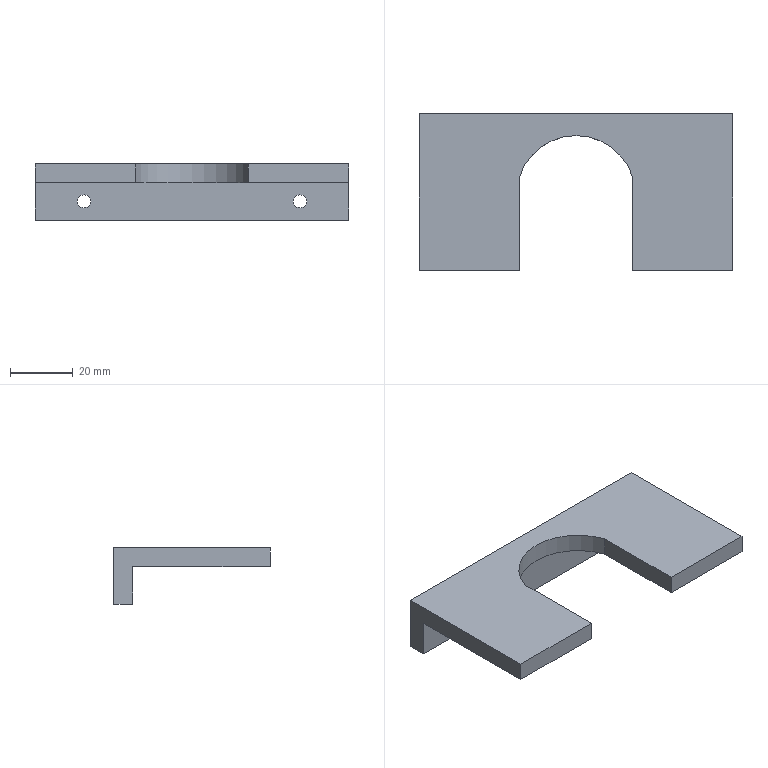Part | STEP file | Tube locking block SGN-6-04 | 1 solid | 16 faces | box 100 x 50 x 18 mm | volume 28496 mm3 | plane 11 | cylinder 5 | commonest cylinder face diameters 4.2 x4 38 x1
STEP:
#1=CARTESIAN_POINT('',(0.,0.,0.));
#2=DIRECTION('',(0.,0.,1.));
#3=DIRECTION('',(1.,0.,0.));
#4=AXIS2_PLACEMENT_3D('',#1,#2,#3);
#5=CARTESIAN_POINT('',(-34.5,19.,-3.9));
#6=VERTEX_POINT('',#5);
#7=CARTESIAN_POINT('',(-34.5,25.,-3.9));
#8=VERTEX_POINT('',#7);
#9=CARTESIAN_POINT('',(-34.5,25.,-3.9));
#10=DIRECTION('',(0.,1.,0.));
#11=VECTOR('',#10,1.);
#12=LINE('',#9,#11);
#13=CARTESIAN_POINT('',(-34.5,25.,-6.));
#14=DIRECTION('',(0.,1.,0.));
#15=DIRECTION('',(0.,0.,1.));
#16=AXIS2_PLACEMENT_3D('',#13,#14,#15);
#17=CYLINDRICAL_SURFACE('',#16,2.1);
#18=CARTESIAN_POINT('',(6.283,0.));
#19=DIRECTION('',(0.,1.));
#20=VECTOR('',#19,1.);
#21=LINE('',#18,#20);
#22=(GEOMETRIC_REPRESENTATION_CONTEXT(2)PARAMETRIC_REPRESENTATION_CONTEXT()REPRESENTATION_CONTEXT('',''));
#23=DEFINITIONAL_REPRESENTATION('',(#21),#22);
#24=PCURVE('',#17,#23);
#25=CARTESIAN_POINT('',(-34.5,25.,-6.));
#26=DIRECTION('',(0.,1.,0.));
#27=DIRECTION('',(0.,0.,1.));
#28=AXIS2_PLACEMENT_3D('',#25,#26,#27);
#29=CYLINDRICAL_SURFACE('',#28,2.1);
#30=CARTESIAN_POINT('',(0.,0.));
#31=DIRECTION('',(0.,1.));
#32=VECTOR('',#31,1.);
#33=LINE('',#30,#32);
#34=(GEOMETRIC_REPRESENTATION_CONTEXT(2)PARAMETRIC_REPRESENTATION_CONTEXT()REPRESENTATION_CONTEXT('',''));
#35=DEFINITIONAL_REPRESENTATION('',(#33),#34);
#36=PCURVE('',#29,#35);
#37=SURFACE_CURVE('',#12,(#24,#36),.PCURVE_S1.);
#38=EDGE_CURVE('',#6,#8,#37,.T.);
#39=ORIENTED_EDGE('',*,*,#38,.T.);
#40=CARTESIAN_POINT('',(-34.5,25.,-8.1));
#41=VERTEX_POINT('',#40);
#42=CARTESIAN_POINT('',(-34.5,25.,-6.));
#43=DIRECTION('',(0.,1.,0.));
#44=DIRECTION('',(0.,0.,1.));
#45=AXIS2_PLACEMENT_3D('',#42,#43,#44);
#46=CIRCLE('',#45,2.1);
#47=CARTESIAN_POINT('',(0.,0.));
#48=DIRECTION('',(1.,0.));
#49=VECTOR('',#48,1.);
#50=LINE('',#47,#49);
#51=(GEOMETRIC_REPRESENTATION_CONTEXT(2)PARAMETRIC_REPRESENTATION_CONTEXT()REPRESENTATION_CONTEXT('',''));
#52=DEFINITIONAL_REPRESENTATION('',(#50),#51);
#53=PCURVE('',#17,#52);
#54=CARTESIAN_POINT('',(-50.,25.,6.));
#55=DIRECTION('',(0.,-1.,0.));
#56=DIRECTION('',(1.,0.,0.));
#57=AXIS2_PLACEMENT_3D('',#54,#55,#56);
#58=PLANE('',#57);
#59=CARTESIAN_POINT('',(15.5,-9.9));
#60=CARTESIAN_POINT('',(19.137,-9.9));
#61=CARTESIAN_POINT('',(17.319,-13.05));
#62=CARTESIAN_POINT('',(15.5,-16.2));
#63=CARTESIAN_POINT('',(13.681,-13.05));
#64=CARTESIAN_POINT('',(11.863,-9.9));
#65=CARTESIAN_POINT('',(15.5,-9.9));
#66=(BOUNDED_CURVE()B_SPLINE_CURVE(2,(#59,#60,#61,#62,#63,#64,#65),.UNSPECIFIED.,.T.,.F.)B_SPLINE_CURVE_WITH_KNOTS((1,2,2,2,2,1),(-2.094,0.,2.094,4.189,6.283,8.378),.UNSPECIFIED.)CURVE()GEOMETRIC_REPRESENTATION_ITEM()RATIONAL_B_SPLINE_CURVE((1.,0.5,1.,0.5,1.,0.5,1.))REPRESENTATION_ITEM(''));
#67=(GEOMETRIC_REPRESENTATION_CONTEXT(2)PARAMETRIC_REPRESENTATION_CONTEXT()REPRESENTATION_CONTEXT('',''));
#68=DEFINITIONAL_REPRESENTATION('',(#66),#67);
#69=PCURVE('',#58,#68);
#70=SURFACE_CURVE('',#46,(#53,#69),.PCURVE_S1.);
#71=EDGE_CURVE('',#41,#8,#70,.T.);
#72=ORIENTED_EDGE('',*,*,#71,.F.);
#73=CARTESIAN_POINT('',(-34.5,19.,-8.1));
#74=VERTEX_POINT('',#73);
#75=CARTESIAN_POINT('',(-34.5,25.,-8.1));
#76=DIRECTION('',(0.,1.,0.));
#77=VECTOR('',#76,1.);
#78=LINE('',#75,#77);
#79=CARTESIAN_POINT('',(3.142,0.));
#80=DIRECTION('',(0.,1.));
#81=VECTOR('',#80,1.);
#82=LINE('',#79,#81);
#83=(GEOMETRIC_REPRESENTATION_CONTEXT(2)PARAMETRIC_REPRESENTATION_CONTEXT()REPRESENTATION_CONTEXT('',''));
#84=DEFINITIONAL_REPRESENTATION('',(#82),#83);
#85=PCURVE('',#17,#84);
#86=CARTESIAN_POINT('',(3.142,0.));
#87=DIRECTION('',(0.,1.));
#88=VECTOR('',#87,1.);
#89=LINE('',#86,#88);
#90=(GEOMETRIC_REPRESENTATION_CONTEXT(2)PARAMETRIC_REPRESENTATION_CONTEXT()REPRESENTATION_CONTEXT('',''));
#91=DEFINITIONAL_REPRESENTATION('',(#89),#90);
#92=PCURVE('',#29,#91);
#93=SURFACE_CURVE('',#78,(#85,#92),.PCURVE_S1.);
#94=EDGE_CURVE('',#74,#41,#93,.T.);
#95=ORIENTED_EDGE('',*,*,#94,.F.);
#96=CARTESIAN_POINT('',(-34.5,19.,-6.));
#97=DIRECTION('',(0.,1.,0.));
#98=DIRECTION('',(0.,0.,1.));
#99=AXIS2_PLACEMENT_3D('',#96,#97,#98);
#100=CIRCLE('',#99,2.1);
#101=CARTESIAN_POINT('',(0.,-6.));
#102=DIRECTION('',(1.,0.));
#103=VECTOR('',#102,1.);
#104=LINE('',#101,#103);
#105=(GEOMETRIC_REPRESENTATION_CONTEXT(2)PARAMETRIC_REPRESENTATION_CONTEXT()REPRESENTATION_CONTEXT('',''));
#106=DEFINITIONAL_REPRESENTATION('',(#104),#105);
#107=PCURVE('',#17,#106);
#108=CARTESIAN_POINT('',(50.,19.,-12.));
#109=DIRECTION('',(0.,1.,0.));
#110=DIRECTION('',(0.,0.,1.));
#111=AXIS2_PLACEMENT_3D('',#108,#109,#110);
#112=PLANE('',#111);
#113=CARTESIAN_POINT('',(6.,-84.5));
#114=DIRECTION('',(1.,0.));
#115=AXIS2_PLACEMENT_2D('',#113,#114);
#116=CIRCLE('',#115,2.1);
#117=(GEOMETRIC_REPRESENTATION_CONTEXT(2)PARAMETRIC_REPRESENTATION_CONTEXT()REPRESENTATION_CONTEXT('',''));
#118=DEFINITIONAL_REPRESENTATION('',(#116),#117);
#119=PCURVE('',#112,#118);
#120=SURFACE_CURVE('',#100,(#107,#119),.PCURVE_S1.);
#121=EDGE_CURVE('',#74,#6,#120,.T.);
#122=ORIENTED_EDGE('',*,*,#121,.T.);
#123=EDGE_LOOP('',(#39,#72,#95,#122));
#124=FACE_BOUND('',#123,.F.);
#125=ADVANCED_FACE('',(#124),#17,.F.);
#126=CARTESIAN_POINT('',(34.5,19.,-3.9));
#127=VERTEX_POINT('',#126);
#128=CARTESIAN_POINT('',(34.5,25.,-3.9));
#129=VERTEX_POINT('',#128);
#130=CARTESIAN_POINT('',(34.5,25.,-3.9));
#131=DIRECTION('',(0.,1.,0.));
#132=VECTOR('',#131,1.);
#133=LINE('',#130,#132);
#134=CARTESIAN_POINT('',(34.5,25.,-6.));
#135=DIRECTION('',(0.,1.,0.));
#136=DIRECTION('',(0.,0.,1.));
#137=AXIS2_PLACEMENT_3D('',#134,#135,#136);
#138=CYLINDRICAL_SURFACE('',#137,2.1);
#139=CARTESIAN_POINT('',(6.283,0.));
#140=DIRECTION('',(0.,1.));
#141=VECTOR('',#140,1.);
#142=LINE('',#139,#141);
#143=(GEOMETRIC_REPRESENTATION_CONTEXT(2)PARAMETRIC_REPRESENTATION_CONTEXT()REPRESENTATION_CONTEXT('',''));
#144=DEFINITIONAL_REPRESENTATION('',(#142),#143);
#145=PCURVE('',#138,#144);
#146=CARTESIAN_POINT('',(34.5,25.,-6.));
#147=DIRECTION('',(0.,1.,0.));
#148=DIRECTION('',(0.,0.,1.));
#149=AXIS2_PLACEMENT_3D('',#146,#147,#148);
#150=CYLINDRICAL_SURFACE('',#149,2.1);
#151=CARTESIAN_POINT('',(0.,0.));
#152=DIRECTION('',(0.,1.));
#153=VECTOR('',#152,1.);
#154=LINE('',#151,#153);
#155=(GEOMETRIC_REPRESENTATION_CONTEXT(2)PARAMETRIC_REPRESENTATION_CONTEXT()REPRESENTATION_CONTEXT('',''));
#156=DEFINITIONAL_REPRESENTATION('',(#154),#155);
#157=PCURVE('',#150,#156);
#158=SURFACE_CURVE('',#133,(#145,#157),.PCURVE_S1.);
#159=EDGE_CURVE('',#127,#129,#158,.T.);
#160=ORIENTED_EDGE('',*,*,#159,.T.);
#161=CARTESIAN_POINT('',(34.5,25.,-8.1));
#162=VERTEX_POINT('',#161);
#163=CARTESIAN_POINT('',(34.5,25.,-6.));
#164=DIRECTION('',(0.,1.,0.));
#165=DIRECTION('',(0.,0.,1.));
#166=AXIS2_PLACEMENT_3D('',#163,#164,#165);
#167=CIRCLE('',#166,2.1);
#168=CARTESIAN_POINT('',(0.,0.));
#169=DIRECTION('',(1.,0.));
#170=VECTOR('',#169,1.);
#171=LINE('',#168,#170);
#172=(GEOMETRIC_REPRESENTATION_CONTEXT(2)PARAMETRIC_REPRESENTATION_CONTEXT()REPRESENTATION_CONTEXT('',''));
#173=DEFINITIONAL_REPRESENTATION('',(#171),#172);
#174=PCURVE('',#138,#173);
#175=CARTESIAN_POINT('',(84.5,-9.9));
#176=CARTESIAN_POINT('',(88.137,-9.9));
#177=CARTESIAN_POINT('',(86.319,-13.05));
#178=CARTESIAN_POINT('',(84.5,-16.2));
#179=CARTESIAN_POINT('',(82.681,-13.05));
#180=CARTESIAN_POINT('',(80.863,-9.9));
#181=CARTESIAN_POINT('',(84.5,-9.9));
#182=(BOUNDED_CURVE()B_SPLINE_CURVE(2,(#175,#176,#177,#178,#179,#180,#181),.UNSPECIFIED.,.T.,.F.)B_SPLINE_CURVE_WITH_KNOTS((1,2,2,2,2,1),(-2.094,0.,2.094,4.189,6.283,8.378),.UNSPECIFIED.)CURVE()GEOMETRIC_REPRESENTATION_ITEM()RATIONAL_B_SPLINE_CURVE((1.,0.5,1.,0.5,1.,0.5,1.))REPRESENTATION_ITEM(''));
#183=(GEOMETRIC_REPRESENTATION_CONTEXT(2)PARAMETRIC_REPRESENTATION_CONTEXT()REPRESENTATION_CONTEXT('',''));
#184=DEFINITIONAL_REPRESENTATION('',(#182),#183);
#185=PCURVE('',#58,#184);
#186=SURFACE_CURVE('',#167,(#174,#185),.PCURVE_S1.);
#187=EDGE_CURVE('',#162,#129,#186,.T.);
#188=ORIENTED_EDGE('',*,*,#187,.F.);
#189=CARTESIAN_POINT('',(34.5,19.,-8.1));
#190=VERTEX_POINT('',#189);
#191=CARTESIAN_POINT('',(34.5,25.,-8.1));
#192=DIRECTION('',(0.,1.,0.));
#193=VECTOR('',#192,1.);
#194=LINE('',#191,#193);
#195=CARTESIAN_POINT('',(3.142,0.));
#196=DIRECTION('',(0.,1.));
#197=VECTOR('',#196,1.);
#198=LINE('',#195,#197);
#199=(GEOMETRIC_REPRESENTATION_CONTEXT(2)PARAMETRIC_REPRESENTATION_CONTEXT()REPRESENTATION_CONTEXT('',''));
#200=DEFINITIONAL_REPRESENTATION('',(#198),#199);
#201=PCURVE('',#138,#200);
#202=CARTESIAN_POINT('',(3.142,0.));
#203=DIRECTION('',(0.,1.));
#204=VECTOR('',#203,1.);
#205=LINE('',#202,#204);
#206=(GEOMETRIC_REPRESENTATION_CONTEXT(2)PARAMETRIC_REPRESENTATION_CONTEXT()REPRESENTATION_CONTEXT('',''));
#207=DEFINITIONAL_REPRESENTATION('',(#205),#206);
#208=PCURVE('',#150,#207);
#209=SURFACE_CURVE('',#194,(#201,#208),.PCURVE_S1.);
#210=EDGE_CURVE('',#190,#162,#209,.T.);
#211=ORIENTED_EDGE('',*,*,#210,.F.);
#212=CARTESIAN_POINT('',(34.5,19.,-6.));
#213=DIRECTION('',(0.,1.,0.));
#214=DIRECTION('',(0.,0.,1.));
#215=AXIS2_PLACEMENT_3D('',#212,#213,#214);
#216=CIRCLE('',#215,2.1);
#217=CARTESIAN_POINT('',(0.,-6.));
#218=DIRECTION('',(1.,0.));
#219=VECTOR('',#218,1.);
#220=LINE('',#217,#219);
#221=(GEOMETRIC_REPRESENTATION_CONTEXT(2)PARAMETRIC_REPRESENTATION_CONTEXT()REPRESENTATION_CONTEXT('',''));
#222=DEFINITIONAL_REPRESENTATION('',(#220),#221);
#223=PCURVE('',#138,#222);
#224=CARTESIAN_POINT('',(6.,-15.5));
#225=DIRECTION('',(1.,0.));
#226=AXIS2_PLACEMENT_2D('',#224,#225);
#227=CIRCLE('',#226,2.1);
#228=(GEOMETRIC_REPRESENTATION_CONTEXT(2)PARAMETRIC_REPRESENTATION_CONTEXT()REPRESENTATION_CONTEXT('',''));
#229=DEFINITIONAL_REPRESENTATION('',(#227),#228);
#230=PCURVE('',#112,#229);
#231=SURFACE_CURVE('',#216,(#223,#230),.PCURVE_S1.);
#232=EDGE_CURVE('',#190,#127,#231,.T.);
#233=ORIENTED_EDGE('',*,*,#232,.T.);
#234=EDGE_LOOP('',(#160,#188,#211,#233));
#235=FACE_BOUND('',#234,.F.);
#236=ADVANCED_FACE('',(#235),#138,.F.);
#237=CARTESIAN_POINT('',(18.,-25.,6.));
#238=VERTEX_POINT('',#237);
#239=CARTESIAN_POINT('',(50.,-25.,6.));
#240=VERTEX_POINT('',#239);
#241=CARTESIAN_POINT('',(-50.,-25.,6.));
#242=DIRECTION('',(1.,0.,0.));
#243=VECTOR('',#242,1.);
#244=LINE('',#241,#243);
#245=CARTESIAN_POINT('',(-50.,-25.,6.));
#246=DIRECTION('',(0.,1.,0.));
#247=DIRECTION('',(0.,0.,1.));
#248=AXIS2_PLACEMENT_3D('',#245,#246,#247);
#249=PLANE('',#248);
#250=CARTESIAN_POINT('',(0.,0.));
#251=DIRECTION('',(0.,1.));
#252=VECTOR('',#251,1.);
#253=LINE('',#250,#252);
#254=(GEOMETRIC_REPRESENTATION_CONTEXT(2)PARAMETRIC_REPRESENTATION_CONTEXT()REPRESENTATION_CONTEXT('',''));
#255=DEFINITIONAL_REPRESENTATION('',(#253),#254);
#256=PCURVE('',#249,#255);
#257=CARTESIAN_POINT('',(0.,0.,6.));
#258=DIRECTION('',(0.,0.,-1.));
#259=DIRECTION('',(-1.,0.,0.));
#260=AXIS2_PLACEMENT_3D('',#257,#258,#259);
#261=PLANE('',#260);
#262=CARTESIAN_POINT('',(50.,-25.));
#263=DIRECTION('',(-1.,0.));
#264=VECTOR('',#263,1.);
#265=LINE('',#262,#264);
#266=(GEOMETRIC_REPRESENTATION_CONTEXT(2)PARAMETRIC_REPRESENTATION_CONTEXT()REPRESENTATION_CONTEXT('',''));
#267=DEFINITIONAL_REPRESENTATION('',(#265),#266);
#268=PCURVE('',#261,#267);
#269=SURFACE_CURVE('',#244,(#256,#268),.PCURVE_S1.);
#270=EDGE_CURVE('',#238,#240,#269,.T.);
#271=ORIENTED_EDGE('',*,*,#270,.F.);
#272=CARTESIAN_POINT('',(18.,-25.,0.));
#273=VERTEX_POINT('',#272);
#274=CARTESIAN_POINT('',(18.,-25.,6.));
#275=DIRECTION('',(0.,0.,-1.));
#276=VECTOR('',#275,1.);
#277=LINE('',#274,#276);
#278=CARTESIAN_POINT('',(0.,68.));
#279=DIRECTION('',(-1.,0.));
#280=VECTOR('',#279,1.);
#281=LINE('',#278,#280);
#282=(GEOMETRIC_REPRESENTATION_CONTEXT(2)PARAMETRIC_REPRESENTATION_CONTEXT()REPRESENTATION_CONTEXT('',''));
#283=DEFINITIONAL_REPRESENTATION('',(#281),#282);
#284=PCURVE('',#249,#283);
#285=CARTESIAN_POINT('',(18.,5.089,0.));
#286=DIRECTION('',(1.,0.,0.));
#287=DIRECTION('',(0.,0.,-1.));
#288=AXIS2_PLACEMENT_3D('',#285,#286,#287);
#289=PLANE('',#288);
#290=CARTESIAN_POINT('',(-6.,-30.089));
#291=DIRECTION('',(1.,0.));
#292=VECTOR('',#291,1.);
#293=LINE('',#290,#292);
#294=(GEOMETRIC_REPRESENTATION_CONTEXT(2)PARAMETRIC_REPRESENTATION_CONTEXT()REPRESENTATION_CONTEXT('',''));
#295=DEFINITIONAL_REPRESENTATION('',(#293),#294);
#296=PCURVE('',#289,#295);
#297=SURFACE_CURVE('',#277,(#284,#296),.PCURVE_S1.);
#298=EDGE_CURVE('',#238,#273,#297,.T.);
#299=ORIENTED_EDGE('',*,*,#298,.T.);
#300=CARTESIAN_POINT('',(50.,-25.,0.));
#301=VERTEX_POINT('',#300);
#302=CARTESIAN_POINT('',(-50.,-25.,0.));
#303=DIRECTION('',(1.,0.,0.));
#304=VECTOR('',#303,1.);
#305=LINE('',#302,#304);
#306=CARTESIAN_POINT('',(-6.,0.));
#307=DIRECTION('',(0.,1.));
#308=VECTOR('',#307,1.);
#309=LINE('',#306,#308);
#310=(GEOMETRIC_REPRESENTATION_CONTEXT(2)PARAMETRIC_REPRESENTATION_CONTEXT()REPRESENTATION_CONTEXT('',''));
#311=DEFINITIONAL_REPRESENTATION('',(#309),#310);
#312=PCURVE('',#249,#311);
#313=CARTESIAN_POINT('',(0.,0.,0.));
#314=DIRECTION('',(0.,0.,-1.));
#315=DIRECTION('',(-1.,0.,0.));
#316=AXIS2_PLACEMENT_3D('',#313,#314,#315);
#317=PLANE('',#316);
#318=CARTESIAN_POINT('',(50.,-25.));
#319=DIRECTION('',(-1.,0.));
#320=VECTOR('',#319,1.);
#321=LINE('',#318,#320);
#322=(GEOMETRIC_REPRESENTATION_CONTEXT(2)PARAMETRIC_REPRESENTATION_CONTEXT()REPRESENTATION_CONTEXT('',''));
#323=DEFINITIONAL_REPRESENTATION('',(#321),#322);
#324=PCURVE('',#317,#323);
#325=SURFACE_CURVE('',#305,(#312,#324),.PCURVE_S1.);
#326=EDGE_CURVE('',#273,#301,#325,.T.);
#327=ORIENTED_EDGE('',*,*,#326,.T.);
#328=CARTESIAN_POINT('',(50.,-25.,6.));
#329=DIRECTION('',(0.,0.,-1.));
#330=VECTOR('',#329,1.);
#331=LINE('',#328,#330);
#332=CARTESIAN_POINT('',(0.,100.));
#333=DIRECTION('',(-1.,0.));
#334=VECTOR('',#333,1.);
#335=LINE('',#332,#334);
#336=(GEOMETRIC_REPRESENTATION_CONTEXT(2)PARAMETRIC_REPRESENTATION_CONTEXT()REPRESENTATION_CONTEXT('',''));
#337=DEFINITIONAL_REPRESENTATION('',(#335),#336);
#338=PCURVE('',#249,#337);
#339=CARTESIAN_POINT('',(50.,-25.,6.));
#340=DIRECTION('',(-1.,0.,0.));
#341=DIRECTION('',(0.,0.,1.));
#342=AXIS2_PLACEMENT_3D('',#339,#340,#341);
#343=PLANE('',#342);
#344=CARTESIAN_POINT('',(0.,0.));
#345=DIRECTION('',(-1.,0.));
#346=VECTOR('',#345,1.);
#347=LINE('',#344,#346);
#348=(GEOMETRIC_REPRESENTATION_CONTEXT(2)PARAMETRIC_REPRESENTATION_CONTEXT()REPRESENTATION_CONTEXT('',''));
#349=DEFINITIONAL_REPRESENTATION('',(#347),#348);
#350=PCURVE('',#343,#349);
#351=SURFACE_CURVE('',#331,(#338,#350),.PCURVE_S1.);
#352=EDGE_CURVE('',#240,#301,#351,.T.);
#353=ORIENTED_EDGE('',*,*,#352,.F.);
#354=EDGE_LOOP('',(#271,#299,#327,#353));
#355=FACE_BOUND('',#354,.T.);
#356=ADVANCED_FACE('',(#355),#249,.F.);
#357=CARTESIAN_POINT('',(50.,19.,0.));
#358=VERTEX_POINT('',#357);
#359=CARTESIAN_POINT('',(50.,-25.,0.));
#360=DIRECTION('',(0.,1.,0.));
#361=VECTOR('',#360,1.);
#362=LINE('',#359,#361);
#363=CARTESIAN_POINT('',(-6.,0.));
#364=DIRECTION('',(0.,1.));
#365=VECTOR('',#364,1.);
#366=LINE('',#363,#365);
#367=(GEOMETRIC_REPRESENTATION_CONTEXT(2)PARAMETRIC_REPRESENTATION_CONTEXT()REPRESENTATION_CONTEXT('',''));
#368=DEFINITIONAL_REPRESENTATION('',(#366),#367);
#369=PCURVE('',#343,#368);
#370=CARTESIAN_POINT('',(-50.,-25.));
#371=DIRECTION('',(0.,1.));
#372=VECTOR('',#371,1.);
#373=LINE('',#370,#372);
#374=(GEOMETRIC_REPRESENTATION_CONTEXT(2)PARAMETRIC_REPRESENTATION_CONTEXT()REPRESENTATION_CONTEXT('',''));
#375=DEFINITIONAL_REPRESENTATION('',(#373),#374);
#376=PCURVE('',#317,#375);
#377=SURFACE_CURVE('',#362,(#369,#376),.PCURVE_S1.);
#378=EDGE_CURVE('',#301,#358,#377,.T.);
#379=ORIENTED_EDGE('',*,*,#378,.T.);
#380=CARTESIAN_POINT('',(50.,19.,-12.));
#381=VERTEX_POINT('',#380);
#382=CARTESIAN_POINT('',(50.,19.,-12.));
#383=DIRECTION('',(0.,0.,1.));
#384=VECTOR('',#383,1.);
#385=LINE('',#382,#384);
#386=CARTESIAN_POINT('',(-18.,44.));
#387=DIRECTION('',(1.,0.));
#388=VECTOR('',#387,1.);
#389=LINE('',#386,#388);
#390=(GEOMETRIC_REPRESENTATION_CONTEXT(2)PARAMETRIC_REPRESENTATION_CONTEXT()REPRESENTATION_CONTEXT('',''));
#391=DEFINITIONAL_REPRESENTATION('',(#389),#390);
#392=PCURVE('',#343,#391);
#393=CARTESIAN_POINT('',(0.,0.));
#394=DIRECTION('',(1.,0.));
#395=VECTOR('',#394,1.);
#396=LINE('',#393,#395);
#397=(GEOMETRIC_REPRESENTATION_CONTEXT(2)PARAMETRIC_REPRESENTATION_CONTEXT()REPRESENTATION_CONTEXT('',''));
#398=DEFINITIONAL_REPRESENTATION('',(#396),#397);
#399=PCURVE('',#112,#398);
#400=SURFACE_CURVE('',#385,(#392,#399),.PCURVE_S1.);
#401=EDGE_CURVE('',#381,#358,#400,.T.);
#402=ORIENTED_EDGE('',*,*,#401,.F.);
#403=CARTESIAN_POINT('',(50.,25.,-12.));
#404=VERTEX_POINT('',#403);
#405=CARTESIAN_POINT('',(50.,25.,-12.));
#406=DIRECTION('',(0.,-1.,0.));
#407=VECTOR('',#406,1.);
#408=LINE('',#405,#407);
#409=CARTESIAN_POINT('',(-18.,50.));
#410=DIRECTION('',(0.,-1.));
#411=VECTOR('',#410,1.);
#412=LINE('',#409,#411);
#413=(GEOMETRIC_REPRESENTATION_CONTEXT(2)PARAMETRIC_REPRESENTATION_CONTEXT()REPRESENTATION_CONTEXT('',''));
#414=DEFINITIONAL_REPRESENTATION('',(#412),#413);
#415=PCURVE('',#343,#414);
#416=CARTESIAN_POINT('',(0.,0.,-12.));
#417=DIRECTION('',(0.,0.,-1.));
#418=DIRECTION('',(-1.,0.,0.));
#419=AXIS2_PLACEMENT_3D('',#416,#417,#418);
#420=PLANE('',#419);
#421=CARTESIAN_POINT('',(-50.,25.));
#422=DIRECTION('',(0.,-1.));
#423=VECTOR('',#422,1.);
#424=LINE('',#421,#423);
#425=(GEOMETRIC_REPRESENTATION_CONTEXT(2)PARAMETRIC_REPRESENTATION_CONTEXT()REPRESENTATION_CONTEXT('',''));
#426=DEFINITIONAL_REPRESENTATION('',(#424),#425);
#427=PCURVE('',#420,#426);
#428=SURFACE_CURVE('',#408,(#415,#427),.PCURVE_S1.);
#429=EDGE_CURVE('',#404,#381,#428,.T.);
#430=ORIENTED_EDGE('',*,*,#429,.F.);
#431=CARTESIAN_POINT('',(50.,25.,6.));
#432=VERTEX_POINT('',#431);
#433=CARTESIAN_POINT('',(50.,25.,6.));
#434=DIRECTION('',(0.,0.,-1.));
#435=VECTOR('',#434,1.);
#436=LINE('',#433,#435);
#437=CARTESIAN_POINT('',(0.,50.));
#438=DIRECTION('',(-1.,0.));
#439=VECTOR('',#438,1.);
#440=LINE('',#437,#439);
#441=(GEOMETRIC_REPRESENTATION_CONTEXT(2)PARAMETRIC_REPRESENTATION_CONTEXT()REPRESENTATION_CONTEXT('',''));
#442=DEFINITIONAL_REPRESENTATION('',(#440),#441);
#443=PCURVE('',#343,#442);
#444=CARTESIAN_POINT('',(100.,0.));
#445=DIRECTION('',(0.,-1.));
#446=VECTOR('',#445,1.);
#447=LINE('',#444,#446);
#448=(GEOMETRIC_REPRESENTATION_CONTEXT(2)PARAMETRIC_REPRESENTATION_CONTEXT()REPRESENTATION_CONTEXT('',''));
#449=DEFINITIONAL_REPRESENTATION('',(#447),#448);
#450=PCURVE('',#58,#449);
#451=SURFACE_CURVE('',#436,(#443,#450),.PCURVE_S1.);
#452=EDGE_CURVE('',#432,#404,#451,.T.);
#453=ORIENTED_EDGE('',*,*,#452,.F.);
#454=CARTESIAN_POINT('',(50.,-25.,6.));
#455=DIRECTION('',(0.,1.,0.));
#456=VECTOR('',#455,1.);
#457=LINE('',#454,#456);
#458=CARTESIAN_POINT('',(0.,0.));
#459=DIRECTION('',(0.,1.));
#460=VECTOR('',#459,1.);
#461=LINE('',#458,#460);
#462=(GEOMETRIC_REPRESENTATION_CONTEXT(2)PARAMETRIC_REPRESENTATION_CONTEXT()REPRESENTATION_CONTEXT('',''));
#463=DEFINITIONAL_REPRESENTATION('',(#461),#462);
#464=PCURVE('',#343,#463);
#465=CARTESIAN_POINT('',(-50.,-25.));
#466=DIRECTION('',(0.,1.));
#467=VECTOR('',#466,1.);
#468=LINE('',#465,#467);
#469=(GEOMETRIC_REPRESENTATION_CONTEXT(2)PARAMETRIC_REPRESENTATION_CONTEXT()REPRESENTATION_CONTEXT('',''));
#470=DEFINITIONAL_REPRESENTATION('',(#468),#469);
#471=PCURVE('',#261,#470);
#472=SURFACE_CURVE('',#457,(#464,#471),.PCURVE_S1.);
#473=EDGE_CURVE('',#240,#432,#472,.T.);
#474=ORIENTED_EDGE('',*,*,#473,.F.);
#475=ORIENTED_EDGE('',*,*,#352,.T.);
#476=EDGE_LOOP('',(#379,#402,#430,#453,#474,#475));
#477=FACE_BOUND('',#476,.T.);
#478=ADVANCED_FACE('',(#477),#343,.F.);
#479=CARTESIAN_POINT('',(-34.5,25.,-6.));
#480=DIRECTION('',(0.,1.,0.));
#481=DIRECTION('',(0.,0.,1.));
#482=AXIS2_PLACEMENT_3D('',#479,#480,#481);
#483=CIRCLE('',#482,2.1);
#484=CARTESIAN_POINT('',(15.5,-9.9));
#485=CARTESIAN_POINT('',(19.137,-9.9));
#486=CARTESIAN_POINT('',(17.319,-13.05));
#487=CARTESIAN_POINT('',(15.5,-16.2));
#488=CARTESIAN_POINT('',(13.681,-13.05));
#489=CARTESIAN_POINT('',(11.863,-9.9));
#490=CARTESIAN_POINT('',(15.5,-9.9));
#491=(BOUNDED_CURVE()B_SPLINE_CURVE(2,(#484,#485,#486,#487,#488,#489,#490),.UNSPECIFIED.,.T.,.F.)B_SPLINE_CURVE_WITH_KNOTS((1,2,2,2,2,1),(-2.094,0.,2.094,4.189,6.283,8.378),.UNSPECIFIED.)CURVE()GEOMETRIC_REPRESENTATION_ITEM()RATIONAL_B_SPLINE_CURVE((1.,0.5,1.,0.5,1.,0.5,1.))REPRESENTATION_ITEM(''));
#492=(GEOMETRIC_REPRESENTATION_CONTEXT(2)PARAMETRIC_REPRESENTATION_CONTEXT()REPRESENTATION_CONTEXT('',''));
#493=DEFINITIONAL_REPRESENTATION('',(#491),#492);
#494=PCURVE('',#58,#493);
#495=CARTESIAN_POINT('',(0.,0.));
#496=DIRECTION('',(1.,0.));
#497=VECTOR('',#496,1.);
#498=LINE('',#495,#497);
#499=(GEOMETRIC_REPRESENTATION_CONTEXT(2)PARAMETRIC_REPRESENTATION_CONTEXT()REPRESENTATION_CONTEXT('',''));
#500=DEFINITIONAL_REPRESENTATION('',(#498),#499);
#501=PCURVE('',#29,#500);
#502=SURFACE_CURVE('',#483,(#494,#501),.PCURVE_S1.);
#503=EDGE_CURVE('',#8,#41,#502,.T.);
#504=ORIENTED_EDGE('',*,*,#503,.F.);
#505=ORIENTED_EDGE('',*,*,#71,.F.);
#506=EDGE_LOOP('',(#504,#505));
#507=FACE_BOUND('',#506,.T.);
#508=CARTESIAN_POINT('',(34.5,25.,-6.));
#509=DIRECTION('',(0.,1.,0.));
#510=DIRECTION('',(0.,0.,1.));
#511=AXIS2_PLACEMENT_3D('',#508,#509,#510);
#512=CIRCLE('',#511,2.1);
#513=CARTESIAN_POINT('',(84.5,-9.9));
#514=CARTESIAN_POINT('',(88.137,-9.9));
#515=CARTESIAN_POINT('',(86.319,-13.05));
#516=CARTESIAN_POINT('',(84.5,-16.2));
#517=CARTESIAN_POINT('',(82.681,-13.05));
#518=CARTESIAN_POINT('',(80.863,-9.9));
#519=CARTESIAN_POINT('',(84.5,-9.9));
#520=(BOUNDED_CURVE()B_SPLINE_CURVE(2,(#513,#514,#515,#516,#517,#518,#519),.UNSPECIFIED.,.T.,.F.)B_SPLINE_CURVE_WITH_KNOTS((1,2,2,2,2,1),(-2.094,0.,2.094,4.189,6.283,8.378),.UNSPECIFIED.)CURVE()GEOMETRIC_REPRESENTATION_ITEM()RATIONAL_B_SPLINE_CURVE((1.,0.5,1.,0.5,1.,0.5,1.))REPRESENTATION_ITEM(''));
#521=(GEOMETRIC_REPRESENTATION_CONTEXT(2)PARAMETRIC_REPRESENTATION_CONTEXT()REPRESENTATION_CONTEXT('',''));
#522=DEFINITIONAL_REPRESENTATION('',(#520),#521);
#523=PCURVE('',#58,#522);
#524=CARTESIAN_POINT('',(0.,0.));
#525=DIRECTION('',(1.,0.));
#526=VECTOR('',#525,1.);
#527=LINE('',#524,#526);
#528=(GEOMETRIC_REPRESENTATION_CONTEXT(2)PARAMETRIC_REPRESENTATION_CONTEXT()REPRESENTATION_CONTEXT('',''));
#529=DEFINITIONAL_REPRESENTATION('',(#527),#528);
#530=PCURVE('',#150,#529);
#531=SURFACE_CURVE('',#512,(#523,#530),.PCURVE_S1.);
#532=EDGE_CURVE('',#129,#162,#531,.T.);
#533=ORIENTED_EDGE('',*,*,#532,.F.);
#534=ORIENTED_EDGE('',*,*,#187,.F.);
#535=EDGE_LOOP('',(#533,#534));
#536=FACE_BOUND('',#535,.T.);
#537=ORIENTED_EDGE('',*,*,#452,.T.);
#538=CARTESIAN_POINT('',(-50.,25.,-12.));
#539=VERTEX_POINT('',#538);
#540=CARTESIAN_POINT('',(50.,25.,-12.));
#541=DIRECTION('',(-1.,0.,0.));
#542=VECTOR('',#541,1.);
#543=LINE('',#540,#542);
#544=CARTESIAN_POINT('',(100.,-18.));
#545=DIRECTION('',(-1.,0.));
#546=VECTOR('',#545,1.);
#547=LINE('',#544,#546);
#548=(GEOMETRIC_REPRESENTATION_CONTEXT(2)PARAMETRIC_REPRESENTATION_CONTEXT()REPRESENTATION_CONTEXT('',''));
#549=DEFINITIONAL_REPRESENTATION('',(#547),#548);
#550=PCURVE('',#58,#549);
#551=CARTESIAN_POINT('',(-50.,25.));
#552=DIRECTION('',(1.,0.));
#553=VECTOR('',#552,1.);
#554=LINE('',#551,#553);
#555=(GEOMETRIC_REPRESENTATION_CONTEXT(2)PARAMETRIC_REPRESENTATION_CONTEXT()REPRESENTATION_CONTEXT('',''));
#556=DEFINITIONAL_REPRESENTATION('',(#554),#555);
#557=PCURVE('',#420,#556);
#558=SURFACE_CURVE('',#543,(#550,#557),.PCURVE_S1.);
#559=EDGE_CURVE('',#404,#539,#558,.T.);
#560=ORIENTED_EDGE('',*,*,#559,.T.);
#561=CARTESIAN_POINT('',(-50.,25.,6.));
#562=VERTEX_POINT('',#561);
#563=CARTESIAN_POINT('',(-50.,25.,6.));
#564=DIRECTION('',(0.,0.,-1.));
#565=VECTOR('',#564,1.);
#566=LINE('',#563,#565);
#567=CARTESIAN_POINT('',(0.,0.));
#568=DIRECTION('',(0.,-1.));
#569=VECTOR('',#568,1.);
#570=LINE('',#567,#569);
#571=(GEOMETRIC_REPRESENTATION_CONTEXT(2)PARAMETRIC_REPRESENTATION_CONTEXT()REPRESENTATION_CONTEXT('',''));
#572=DEFINITIONAL_REPRESENTATION('',(#570),#571);
#573=PCURVE('',#58,#572);
#574=CARTESIAN_POINT('',(-50.,-25.,6.));
#575=DIRECTION('',(1.,0.,0.));
#576=DIRECTION('',(0.,0.,-1.));
#577=AXIS2_PLACEMENT_3D('',#574,#575,#576);
#578=PLANE('',#577);
#579=CARTESIAN_POINT('',(0.,50.));
#580=DIRECTION('',(1.,0.));
#581=VECTOR('',#580,1.);
#582=LINE('',#579,#581);
#583=(GEOMETRIC_REPRESENTATION_CONTEXT(2)PARAMETRIC_REPRESENTATION_CONTEXT()REPRESENTATION_CONTEXT('',''));
#584=DEFINITIONAL_REPRESENTATION('',(#582),#583);
#585=PCURVE('',#578,#584);
#586=SURFACE_CURVE('',#566,(#573,#585),.PCURVE_S1.);
#587=EDGE_CURVE('',#562,#539,#586,.T.);
#588=ORIENTED_EDGE('',*,*,#587,.F.);
#589=CARTESIAN_POINT('',(-50.,25.,6.));
#590=DIRECTION('',(-1.,0.,0.));
#591=VECTOR('',#590,1.);
#592=LINE('',#589,#591);
#593=CARTESIAN_POINT('',(0.,0.));
#594=DIRECTION('',(-1.,0.));
#595=VECTOR('',#594,1.);
#596=LINE('',#593,#595);
#597=(GEOMETRIC_REPRESENTATION_CONTEXT(2)PARAMETRIC_REPRESENTATION_CONTEXT()REPRESENTATION_CONTEXT('',''));
#598=DEFINITIONAL_REPRESENTATION('',(#596),#597);
#599=PCURVE('',#58,#598);
#600=CARTESIAN_POINT('',(50.,25.));
#601=DIRECTION('',(1.,0.));
#602=VECTOR('',#601,1.);
#603=LINE('',#600,#602);
#604=(GEOMETRIC_REPRESENTATION_CONTEXT(2)PARAMETRIC_REPRESENTATION_CONTEXT()REPRESENTATION_CONTEXT('',''));
#605=DEFINITIONAL_REPRESENTATION('',(#603),#604);
#606=PCURVE('',#261,#605);
#607=SURFACE_CURVE('',#592,(#599,#606),.PCURVE_S1.);
#608=EDGE_CURVE('',#432,#562,#607,.T.);
#609=ORIENTED_EDGE('',*,*,#608,.F.);
#610=EDGE_LOOP('',(#537,#560,#588,#609));
#611=FACE_BOUND('',#610,.T.);
#612=ADVANCED_FACE('',(#507,#536,#611),#58,.F.);
#613=ORIENTED_EDGE('',*,*,#587,.T.);
#614=CARTESIAN_POINT('',(-50.,19.,-12.));
#615=VERTEX_POINT('',#614);
#616=CARTESIAN_POINT('',(-50.,25.,-12.));
#617=DIRECTION('',(0.,-1.,0.));
#618=VECTOR('',#617,1.);
#619=LINE('',#616,#618);
#620=CARTESIAN_POINT('',(18.,50.));
#621=DIRECTION('',(0.,-1.));
#622=VECTOR('',#621,1.);
#623=LINE('',#620,#622);
#624=(GEOMETRIC_REPRESENTATION_CONTEXT(2)PARAMETRIC_REPRESENTATION_CONTEXT()REPRESENTATION_CONTEXT('',''));
#625=DEFINITIONAL_REPRESENTATION('',(#623),#624);
#626=PCURVE('',#578,#625);
#627=CARTESIAN_POINT('',(50.,25.));
#628=DIRECTION('',(0.,-1.));
#629=VECTOR('',#628,1.);
#630=LINE('',#627,#629);
#631=(GEOMETRIC_REPRESENTATION_CONTEXT(2)PARAMETRIC_REPRESENTATION_CONTEXT()REPRESENTATION_CONTEXT('',''));
#632=DEFINITIONAL_REPRESENTATION('',(#630),#631);
#633=PCURVE('',#420,#632);
#634=SURFACE_CURVE('',#619,(#626,#633),.PCURVE_S1.);
#635=EDGE_CURVE('',#539,#615,#634,.T.);
#636=ORIENTED_EDGE('',*,*,#635,.T.);
#637=CARTESIAN_POINT('',(-50.,19.,0.));
#638=VERTEX_POINT('',#637);
#639=CARTESIAN_POINT('',(-50.,19.,-12.));
#640=DIRECTION('',(0.,0.,1.));
#641=VECTOR('',#640,1.);
#642=LINE('',#639,#641);
#643=CARTESIAN_POINT('',(18.,44.));
#644=DIRECTION('',(-1.,0.));
#645=VECTOR('',#644,1.);
#646=LINE('',#643,#645);
#647=(GEOMETRIC_REPRESENTATION_CONTEXT(2)PARAMETRIC_REPRESENTATION_CONTEXT()REPRESENTATION_CONTEXT('',''));
#648=DEFINITIONAL_REPRESENTATION('',(#646),#647);
#649=PCURVE('',#578,#648);
#650=CARTESIAN_POINT('',(0.,-100.));
#651=DIRECTION('',(1.,0.));
#652=VECTOR('',#651,1.);
#653=LINE('',#650,#652);
#654=(GEOMETRIC_REPRESENTATION_CONTEXT(2)PARAMETRIC_REPRESENTATION_CONTEXT()REPRESENTATION_CONTEXT('',''));
#655=DEFINITIONAL_REPRESENTATION('',(#653),#654);
#656=PCURVE('',#112,#655);
#657=SURFACE_CURVE('',#642,(#649,#656),.PCURVE_S1.);
#658=EDGE_CURVE('',#615,#638,#657,.T.);
#659=ORIENTED_EDGE('',*,*,#658,.T.);
#660=CARTESIAN_POINT('',(-50.,-25.,0.));
#661=VERTEX_POINT('',#660);
#662=CARTESIAN_POINT('',(-50.,-25.,0.));
#663=DIRECTION('',(0.,-1.,0.));
#664=VECTOR('',#663,1.);
#665=LINE('',#662,#664);
#666=CARTESIAN_POINT('',(6.,0.));
#667=DIRECTION('',(0.,-1.));
#668=VECTOR('',#667,1.);
#669=LINE('',#666,#668);
#670=(GEOMETRIC_REPRESENTATION_CONTEXT(2)PARAMETRIC_REPRESENTATION_CONTEXT()REPRESENTATION_CONTEXT('',''));
#671=DEFINITIONAL_REPRESENTATION('',(#669),#670);
#672=PCURVE('',#578,#671);
#673=CARTESIAN_POINT('',(50.,-25.));
#674=DIRECTION('',(0.,-1.));
#675=VECTOR('',#674,1.);
#676=LINE('',#673,#675);
#677=(GEOMETRIC_REPRESENTATION_CONTEXT(2)PARAMETRIC_REPRESENTATION_CONTEXT()REPRESENTATION_CONTEXT('',''));
#678=DEFINITIONAL_REPRESENTATION('',(#676),#677);
#679=PCURVE('',#317,#678);
#680=SURFACE_CURVE('',#665,(#672,#679),.PCURVE_S1.);
#681=EDGE_CURVE('',#638,#661,#680,.T.);
#682=ORIENTED_EDGE('',*,*,#681,.T.);
#683=CARTESIAN_POINT('',(-50.,-25.,6.));
#684=VERTEX_POINT('',#683);
#685=CARTESIAN_POINT('',(-50.,-25.,6.));
#686=DIRECTION('',(0.,0.,-1.));
#687=VECTOR('',#686,1.);
#688=LINE('',#685,#687);
#689=CARTESIAN_POINT('',(0.,0.));
#690=DIRECTION('',(1.,0.));
#691=VECTOR('',#690,1.);
#692=LINE('',#689,#691);
#693=(GEOMETRIC_REPRESENTATION_CONTEXT(2)PARAMETRIC_REPRESENTATION_CONTEXT()REPRESENTATION_CONTEXT('',''));
#694=DEFINITIONAL_REPRESENTATION('',(#692),#693);
#695=PCURVE('',#578,#694);
#696=CARTESIAN_POINT('',(-50.,-25.,6.));
#697=DIRECTION('',(0.,1.,0.));
#698=DIRECTION('',(0.,0.,1.));
#699=AXIS2_PLACEMENT_3D('',#696,#697,#698);
#700=PLANE('',#699);
#701=CARTESIAN_POINT('',(0.,0.));
#702=DIRECTION('',(-1.,0.));
#703=VECTOR('',#702,1.);
#704=LINE('',#701,#703);
#705=(GEOMETRIC_REPRESENTATION_CONTEXT(2)PARAMETRIC_REPRESENTATION_CONTEXT()REPRESENTATION_CONTEXT('',''));
#706=DEFINITIONAL_REPRESENTATION('',(#704),#705);
#707=PCURVE('',#700,#706);
#708=SURFACE_CURVE('',#688,(#695,#707),.PCURVE_S1.);
#709=EDGE_CURVE('',#684,#661,#708,.T.);
#710=ORIENTED_EDGE('',*,*,#709,.F.);
#711=CARTESIAN_POINT('',(-50.,-25.,6.));
#712=DIRECTION('',(0.,-1.,0.));
#713=VECTOR('',#712,1.);
#714=LINE('',#711,#713);
#715=CARTESIAN_POINT('',(0.,0.));
#716=DIRECTION('',(0.,-1.));
#717=VECTOR('',#716,1.);
#718=LINE('',#715,#717);
#719=(GEOMETRIC_REPRESENTATION_CONTEXT(2)PARAMETRIC_REPRESENTATION_CONTEXT()REPRESENTATION_CONTEXT('',''));
#720=DEFINITIONAL_REPRESENTATION('',(#718),#719);
#721=PCURVE('',#578,#720);
#722=CARTESIAN_POINT('',(50.,-25.));
#723=DIRECTION('',(0.,-1.));
#724=VECTOR('',#723,1.);
#725=LINE('',#722,#724);
#726=(GEOMETRIC_REPRESENTATION_CONTEXT(2)PARAMETRIC_REPRESENTATION_CONTEXT()REPRESENTATION_CONTEXT('',''));
#727=DEFINITIONAL_REPRESENTATION('',(#725),#726);
#728=PCURVE('',#261,#727);
#729=SURFACE_CURVE('',#714,(#721,#728),.PCURVE_S1.);
#730=EDGE_CURVE('',#562,#684,#729,.T.);
#731=ORIENTED_EDGE('',*,*,#730,.F.);
#732=EDGE_LOOP('',(#613,#636,#659,#682,#710,#731));
#733=FACE_BOUND('',#732,.T.);
#734=ADVANCED_FACE('',(#733),#578,.F.);
#735=CARTESIAN_POINT('',(-18.,-25.,0.));
#736=VERTEX_POINT('',#735);
#737=CARTESIAN_POINT('',(-50.,-25.,0.));
#738=DIRECTION('',(1.,0.,0.));
#739=VECTOR('',#738,1.);
#740=LINE('',#737,#739);
#741=CARTESIAN_POINT('',(-6.,0.));
#742=DIRECTION('',(0.,1.));
#743=VECTOR('',#742,1.);
#744=LINE('',#741,#743);
#745=(GEOMETRIC_REPRESENTATION_CONTEXT(2)PARAMETRIC_REPRESENTATION_CONTEXT()REPRESENTATION_CONTEXT('',''));
#746=DEFINITIONAL_REPRESENTATION('',(#744),#745);
#747=PCURVE('',#700,#746);
#748=CARTESIAN_POINT('',(50.,-25.));
#749=DIRECTION('',(-1.,0.));
#750=VECTOR('',#749,1.);
#751=LINE('',#748,#750);
#752=(GEOMETRIC_REPRESENTATION_CONTEXT(2)PARAMETRIC_REPRESENTATION_CONTEXT()REPRESENTATION_CONTEXT('',''));
#753=DEFINITIONAL_REPRESENTATION('',(#751),#752);
#754=PCURVE('',#317,#753);
#755=SURFACE_CURVE('',#740,(#747,#754),.PCURVE_S1.);
#756=EDGE_CURVE('',#661,#736,#755,.T.);
#757=ORIENTED_EDGE('',*,*,#756,.T.);
#758=CARTESIAN_POINT('',(-18.,-25.,6.));
#759=VERTEX_POINT('',#758);
#760=CARTESIAN_POINT('',(-18.,-25.,6.));
#761=DIRECTION('',(0.,0.,1.));
#762=VECTOR('',#761,1.);
#763=LINE('',#760,#762);
#764=CARTESIAN_POINT('',(0.,32.));
#765=DIRECTION('',(1.,0.));
#766=VECTOR('',#765,1.);
#767=LINE('',#764,#766);
#768=(GEOMETRIC_REPRESENTATION_CONTEXT(2)PARAMETRIC_REPRESENTATION_CONTEXT()REPRESENTATION_CONTEXT('',''));
#769=DEFINITIONAL_REPRESENTATION('',(#767),#768);
#770=PCURVE('',#700,#769);
#771=CARTESIAN_POINT('',(-18.,5.077,0.));
#772=DIRECTION('',(-1.,0.,0.));
#773=DIRECTION('',(0.,-1.,0.));
#774=AXIS2_PLACEMENT_3D('',#771,#772,#773);
#775=PLANE('',#774);
#776=CARTESIAN_POINT('',(30.077,6.));
#777=DIRECTION('',(0.,1.));
#778=VECTOR('',#777,1.);
#779=LINE('',#776,#778);
#780=(GEOMETRIC_REPRESENTATION_CONTEXT(2)PARAMETRIC_REPRESENTATION_CONTEXT()REPRESENTATION_CONTEXT('',''));
#781=DEFINITIONAL_REPRESENTATION('',(#779),#780);
#782=PCURVE('',#775,#781);
#783=SURFACE_CURVE('',#763,(#770,#782),.PCURVE_S1.);
#784=EDGE_CURVE('',#736,#759,#783,.T.);
#785=ORIENTED_EDGE('',*,*,#784,.T.);
#786=CARTESIAN_POINT('',(-50.,-25.,6.));
#787=DIRECTION('',(1.,0.,0.));
#788=VECTOR('',#787,1.);
#789=LINE('',#786,#788);
#790=CARTESIAN_POINT('',(0.,0.));
#791=DIRECTION('',(0.,1.));
#792=VECTOR('',#791,1.);
#793=LINE('',#790,#792);
#794=(GEOMETRIC_REPRESENTATION_CONTEXT(2)PARAMETRIC_REPRESENTATION_CONTEXT()REPRESENTATION_CONTEXT('',''));
#795=DEFINITIONAL_REPRESENTATION('',(#793),#794);
#796=PCURVE('',#700,#795);
#797=CARTESIAN_POINT('',(50.,-25.));
#798=DIRECTION('',(-1.,0.));
#799=VECTOR('',#798,1.);
#800=LINE('',#797,#799);
#801=(GEOMETRIC_REPRESENTATION_CONTEXT(2)PARAMETRIC_REPRESENTATION_CONTEXT()REPRESENTATION_CONTEXT('',''));
#802=DEFINITIONAL_REPRESENTATION('',(#800),#801);
#803=PCURVE('',#261,#802);
#804=SURFACE_CURVE('',#789,(#796,#803),.PCURVE_S1.);
#805=EDGE_CURVE('',#684,#759,#804,.T.);
#806=ORIENTED_EDGE('',*,*,#805,.F.);
#807=ORIENTED_EDGE('',*,*,#709,.T.);
#808=EDGE_LOOP('',(#757,#785,#806,#807));
#809=FACE_BOUND('',#808,.T.);
#810=ADVANCED_FACE('',(#809),#700,.F.);
#811=CARTESIAN_POINT('',(18.,5.089,6.));
#812=VERTEX_POINT('',#811);
#813=CARTESIAN_POINT('',(-18.,5.077,6.));
#814=VERTEX_POINT('',#813);
#815=CARTESIAN_POINT('',(0.002079,-1.,6.));
#816=DIRECTION('',(0.,0.,1.));
#817=DIRECTION('',(1.,0.,0.));
#818=AXIS2_PLACEMENT_3D('',#815,#816,#817);
#819=CIRCLE('',#818,19.);
#820=CARTESIAN_POINT('',(-19.002,-1.));
#821=CARTESIAN_POINT('',(-19.002,31.909));
#822=CARTESIAN_POINT('',(9.498,15.454));
#823=CARTESIAN_POINT('',(37.998,-1.));
#824=CARTESIAN_POINT('',(9.498,-17.454));
#825=CARTESIAN_POINT('',(-19.002,-33.909));
#826=CARTESIAN_POINT('',(-19.002,-1.));
#827=(BOUNDED_CURVE()B_SPLINE_CURVE(2,(#820,#821,#822,#823,#824,#825,#826),.UNSPECIFIED.,.T.,.F.)B_SPLINE_CURVE_WITH_KNOTS((1,2,2,2,2,1),(-2.094,0.,2.094,4.189,6.283,8.378),.UNSPECIFIED.)CURVE()GEOMETRIC_REPRESENTATION_ITEM()RATIONAL_B_SPLINE_CURVE((1.,0.5,1.,0.5,1.,0.5,1.))REPRESENTATION_ITEM(''));
#828=(GEOMETRIC_REPRESENTATION_CONTEXT(2)PARAMETRIC_REPRESENTATION_CONTEXT()REPRESENTATION_CONTEXT('',''));
#829=DEFINITIONAL_REPRESENTATION('',(#827),#828);
#830=PCURVE('',#261,#829);
#831=CARTESIAN_POINT('',(0.002079,-1.,0.));
#832=DIRECTION('',(0.,0.,1.));
#833=DIRECTION('',(1.,0.,0.));
#834=AXIS2_PLACEMENT_3D('',#831,#832,#833);
#835=CYLINDRICAL_SURFACE('',#834,19.);
#836=CARTESIAN_POINT('',(0.,6.));
#837=DIRECTION('',(1.,0.));
#838=VECTOR('',#837,1.);
#839=LINE('',#836,#838);
#840=(GEOMETRIC_REPRESENTATION_CONTEXT(2)PARAMETRIC_REPRESENTATION_CONTEXT()REPRESENTATION_CONTEXT('',''));
#841=DEFINITIONAL_REPRESENTATION('',(#839),#840);
#842=PCURVE('',#835,#841);
#843=SURFACE_CURVE('',#819,(#830,#842),.PCURVE_S1.);
#844=EDGE_CURVE('',#812,#814,#843,.T.);
#845=ORIENTED_EDGE('',*,*,#844,.F.);
#846=CARTESIAN_POINT('',(18.,5.089,6.));
#847=DIRECTION('',(0.,1.,0.));
#848=VECTOR('',#847,1.);
#849=LINE('',#846,#848);
#850=CARTESIAN_POINT('',(-18.,5.089));
#851=DIRECTION('',(0.,1.));
#852=VECTOR('',#851,1.);
#853=LINE('',#850,#852);
#854=(GEOMETRIC_REPRESENTATION_CONTEXT(2)PARAMETRIC_REPRESENTATION_CONTEXT()REPRESENTATION_CONTEXT('',''));
#855=DEFINITIONAL_REPRESENTATION('',(#853),#854);
#856=PCURVE('',#261,#855);
#857=CARTESIAN_POINT('',(-6.,0.));
#858=DIRECTION('',(0.,1.));
#859=VECTOR('',#858,1.);
#860=LINE('',#857,#859);
#861=(GEOMETRIC_REPRESENTATION_CONTEXT(2)PARAMETRIC_REPRESENTATION_CONTEXT()REPRESENTATION_CONTEXT('',''));
#862=DEFINITIONAL_REPRESENTATION('',(#860),#861);
#863=PCURVE('',#289,#862);
#864=SURFACE_CURVE('',#849,(#856,#863),.PCURVE_S1.);
#865=EDGE_CURVE('',#238,#812,#864,.T.);
#866=ORIENTED_EDGE('',*,*,#865,.F.);
#867=ORIENTED_EDGE('',*,*,#270,.T.);
#868=ORIENTED_EDGE('',*,*,#473,.T.);
#869=ORIENTED_EDGE('',*,*,#608,.T.);
#870=ORIENTED_EDGE('',*,*,#730,.T.);
#871=ORIENTED_EDGE('',*,*,#805,.T.);
#872=CARTESIAN_POINT('',(-18.,5.077,6.));
#873=DIRECTION('',(0.,-1.,0.));
#874=VECTOR('',#873,1.);
#875=LINE('',#872,#874);
#876=CARTESIAN_POINT('',(18.,5.077));
#877=DIRECTION('',(0.,-1.));
#878=VECTOR('',#877,1.);
#879=LINE('',#876,#878);
#880=(GEOMETRIC_REPRESENTATION_CONTEXT(2)PARAMETRIC_REPRESENTATION_CONTEXT()REPRESENTATION_CONTEXT('',''));
#881=DEFINITIONAL_REPRESENTATION('',(#879),#880);
#882=PCURVE('',#261,#881);
#883=CARTESIAN_POINT('',(0.,6.));
#884=DIRECTION('',(1.,0.));
#885=VECTOR('',#884,1.);
#886=LINE('',#883,#885);
#887=(GEOMETRIC_REPRESENTATION_CONTEXT(2)PARAMETRIC_REPRESENTATION_CONTEXT()REPRESENTATION_CONTEXT('',''));
#888=DEFINITIONAL_REPRESENTATION('',(#886),#887);
#889=PCURVE('',#775,#888);
#890=SURFACE_CURVE('',#875,(#882,#889),.PCURVE_S1.);
#891=EDGE_CURVE('',#814,#759,#890,.T.);
#892=ORIENTED_EDGE('',*,*,#891,.F.);
#893=EDGE_LOOP('',(#845,#866,#867,#868,#869,#870,#871,#892));
#894=FACE_BOUND('',#893,.T.);
#895=ADVANCED_FACE('',(#894),#261,.F.);
#896=CARTESIAN_POINT('',(50.,19.,0.));
#897=DIRECTION('',(-1.,0.,0.));
#898=VECTOR('',#897,1.);
#899=LINE('',#896,#898);
#900=CARTESIAN_POINT('',(-50.,19.));
#901=DIRECTION('',(1.,0.));
#902=VECTOR('',#901,1.);
#903=LINE('',#900,#902);
#904=(GEOMETRIC_REPRESENTATION_CONTEXT(2)PARAMETRIC_REPRESENTATION_CONTEXT()REPRESENTATION_CONTEXT('',''));
#905=DEFINITIONAL_REPRESENTATION('',(#903),#904);
#906=PCURVE('',#317,#905);
#907=CARTESIAN_POINT('',(12.,0.));
#908=DIRECTION('',(0.,-1.));
#909=VECTOR('',#908,1.);
#910=LINE('',#907,#909);
#911=(GEOMETRIC_REPRESENTATION_CONTEXT(2)PARAMETRIC_REPRESENTATION_CONTEXT()REPRESENTATION_CONTEXT('',''));
#912=DEFINITIONAL_REPRESENTATION('',(#910),#911);
#913=PCURVE('',#112,#912);
#914=SURFACE_CURVE('',#899,(#906,#913),.PCURVE_S1.);
#915=EDGE_CURVE('',#358,#638,#914,.T.);
#916=ORIENTED_EDGE('',*,*,#915,.F.);
#917=ORIENTED_EDGE('',*,*,#378,.F.);
#918=ORIENTED_EDGE('',*,*,#326,.F.);
#919=CARTESIAN_POINT('',(18.,5.089,0.));
#920=VERTEX_POINT('',#919);
#921=CARTESIAN_POINT('',(18.,0.,0.));
#922=DIRECTION('',(0.,-1.,0.));
#923=VECTOR('',#922,1.);
#924=LINE('',#921,#923);
#925=CARTESIAN_POINT('',(-18.,0.));
#926=DIRECTION('',(0.,-1.));
#927=VECTOR('',#926,1.);
#928=LINE('',#925,#927);
#929=(GEOMETRIC_REPRESENTATION_CONTEXT(2)PARAMETRIC_REPRESENTATION_CONTEXT()REPRESENTATION_CONTEXT('',''));
#930=DEFINITIONAL_REPRESENTATION('',(#928),#929);
#931=PCURVE('',#317,#930);
#932=CARTESIAN_POINT('',(0.,-5.089));
#933=DIRECTION('',(0.,-1.));
#934=VECTOR('',#933,1.);
#935=LINE('',#932,#934);
#936=(GEOMETRIC_REPRESENTATION_CONTEXT(2)PARAMETRIC_REPRESENTATION_CONTEXT()REPRESENTATION_CONTEXT('',''));
#937=DEFINITIONAL_REPRESENTATION('',(#935),#936);
#938=PCURVE('',#289,#937);
#939=SURFACE_CURVE('',#924,(#931,#938),.PCURVE_S1.);
#940=EDGE_CURVE('',#920,#273,#939,.T.);
#941=ORIENTED_EDGE('',*,*,#940,.F.);
#942=CARTESIAN_POINT('',(-18.,5.077,0.));
#943=VERTEX_POINT('',#942);
#944=CARTESIAN_POINT('',(0.002079,-1.,0.));
#945=DIRECTION('',(0.,0.,1.));
#946=DIRECTION('',(1.,0.,0.));
#947=AXIS2_PLACEMENT_3D('',#944,#945,#946);
#948=CIRCLE('',#947,19.);
#949=CARTESIAN_POINT('',(-19.002,-1.));
#950=CARTESIAN_POINT('',(-19.002,31.909));
#951=CARTESIAN_POINT('',(9.498,15.454));
#952=CARTESIAN_POINT('',(37.998,-1.));
#953=CARTESIAN_POINT('',(9.498,-17.454));
#954=CARTESIAN_POINT('',(-19.002,-33.909));
#955=CARTESIAN_POINT('',(-19.002,-1.));
#956=(BOUNDED_CURVE()B_SPLINE_CURVE(2,(#949,#950,#951,#952,#953,#954,#955),.UNSPECIFIED.,.T.,.F.)B_SPLINE_CURVE_WITH_KNOTS((1,2,2,2,2,1),(-2.094,0.,2.094,4.189,6.283,8.378),.UNSPECIFIED.)CURVE()GEOMETRIC_REPRESENTATION_ITEM()RATIONAL_B_SPLINE_CURVE((1.,0.5,1.,0.5,1.,0.5,1.))REPRESENTATION_ITEM(''));
#957=(GEOMETRIC_REPRESENTATION_CONTEXT(2)PARAMETRIC_REPRESENTATION_CONTEXT()REPRESENTATION_CONTEXT('',''));
#958=DEFINITIONAL_REPRESENTATION('',(#956),#957);
#959=PCURVE('',#317,#958);
#960=CARTESIAN_POINT('',(0.,0.));
#961=DIRECTION('',(1.,0.));
#962=VECTOR('',#961,1.);
#963=LINE('',#960,#962);
#964=(GEOMETRIC_REPRESENTATION_CONTEXT(2)PARAMETRIC_REPRESENTATION_CONTEXT()REPRESENTATION_CONTEXT('',''));
#965=DEFINITIONAL_REPRESENTATION('',(#963),#964);
#966=PCURVE('',#835,#965);
#967=SURFACE_CURVE('',#948,(#959,#966),.PCURVE_S1.);
#968=EDGE_CURVE('',#920,#943,#967,.T.);
#969=ORIENTED_EDGE('',*,*,#968,.T.);
#970=CARTESIAN_POINT('',(-18.,5.077,0.));
#971=DIRECTION('',(0.,-1.,0.));
#972=VECTOR('',#971,1.);
#973=LINE('',#970,#972);
#974=CARTESIAN_POINT('',(18.,5.077));
#975=DIRECTION('',(0.,-1.));
#976=VECTOR('',#975,1.);
#977=LINE('',#974,#976);
#978=(GEOMETRIC_REPRESENTATION_CONTEXT(2)PARAMETRIC_REPRESENTATION_CONTEXT()REPRESENTATION_CONTEXT('',''));
#979=DEFINITIONAL_REPRESENTATION('',(#977),#978);
#980=PCURVE('',#317,#979);
#981=CARTESIAN_POINT('',(0.,0.));
#982=DIRECTION('',(1.,0.));
#983=VECTOR('',#982,1.);
#984=LINE('',#981,#983);
#985=(GEOMETRIC_REPRESENTATION_CONTEXT(2)PARAMETRIC_REPRESENTATION_CONTEXT()REPRESENTATION_CONTEXT('',''));
#986=DEFINITIONAL_REPRESENTATION('',(#984),#985);
#987=PCURVE('',#775,#986);
#988=SURFACE_CURVE('',#973,(#980,#987),.PCURVE_S1.);
#989=EDGE_CURVE('',#943,#736,#988,.T.);
#990=ORIENTED_EDGE('',*,*,#989,.T.);
#991=ORIENTED_EDGE('',*,*,#756,.F.);
#992=ORIENTED_EDGE('',*,*,#681,.F.);
#993=EDGE_LOOP('',(#916,#917,#918,#941,#969,#990,#991,#992));
#994=FACE_BOUND('',#993,.T.);
#995=ADVANCED_FACE('',(#994),#317,.T.);
#996=ORIENTED_EDGE('',*,*,#865,.T.);
#997=CARTESIAN_POINT('',(18.,5.089,0.));
#998=DIRECTION('',(0.,0.,1.));
#999=VECTOR('',#998,1.);
#1000=LINE('',#997,#999);
#1001=CARTESIAN_POINT('',(0.,0.));
#1002=DIRECTION('',(-1.,0.));
#1003=VECTOR('',#1002,1.);
#1004=LINE('',#1001,#1003);
#1005=(GEOMETRIC_REPRESENTATION_CONTEXT(2)PARAMETRIC_REPRESENTATION_CONTEXT()REPRESENTATION_CONTEXT('',''));
#1006=DEFINITIONAL_REPRESENTATION('',(#1004),#1005);
#1007=PCURVE('',#289,#1006);
#1008=CARTESIAN_POINT('',(0.3262,0.));
#1009=DIRECTION('',(0.,1.));
#1010=VECTOR('',#1009,1.);
#1011=LINE('',#1008,#1010);
#1012=(GEOMETRIC_REPRESENTATION_CONTEXT(2)PARAMETRIC_REPRESENTATION_CONTEXT()REPRESENTATION_CONTEXT('',''));
#1013=DEFINITIONAL_REPRESENTATION('',(#1011),#1012);
#1014=PCURVE('',#835,#1013);
#1015=SURFACE_CURVE('',#1000,(#1007,#1014),.PCURVE_S1.);
#1016=EDGE_CURVE('',#920,#812,#1015,.T.);
#1017=ORIENTED_EDGE('',*,*,#1016,.F.);
#1018=ORIENTED_EDGE('',*,*,#940,.T.);
#1019=ORIENTED_EDGE('',*,*,#298,.F.);
#1020=EDGE_LOOP('',(#996,#1017,#1018,#1019));
#1021=FACE_BOUND('',#1020,.T.);
#1022=ADVANCED_FACE('',(#1021),#289,.F.);
#1023=ORIENTED_EDGE('',*,*,#989,.F.);
#1024=CARTESIAN_POINT('',(-18.,5.077,0.));
#1025=DIRECTION('',(0.,0.,1.));
#1026=VECTOR('',#1025,1.);
#1027=LINE('',#1024,#1026);
#1028=CARTESIAN_POINT('',(0.,0.));
#1029=DIRECTION('',(0.,1.));
#1030=VECTOR('',#1029,1.);
#1031=LINE('',#1028,#1030);
#1032=(GEOMETRIC_REPRESENTATION_CONTEXT(2)PARAMETRIC_REPRESENTATION_CONTEXT()REPRESENTATION_CONTEXT('',''));
#1033=DEFINITIONAL_REPRESENTATION('',(#1031),#1032);
#1034=PCURVE('',#775,#1033);
#1035=CARTESIAN_POINT('',(2.816,0.));
#1036=DIRECTION('',(0.,1.));
#1037=VECTOR('',#1036,1.);
#1038=LINE('',#1035,#1037);
#1039=(GEOMETRIC_REPRESENTATION_CONTEXT(2)PARAMETRIC_REPRESENTATION_CONTEXT()REPRESENTATION_CONTEXT('',''));
#1040=DEFINITIONAL_REPRESENTATION('',(#1038),#1039);
#1041=PCURVE('',#835,#1040);
#1042=SURFACE_CURVE('',#1027,(#1034,#1041),.PCURVE_S1.);
#1043=EDGE_CURVE('',#943,#814,#1042,.T.);
#1044=ORIENTED_EDGE('',*,*,#1043,.T.);
#1045=ORIENTED_EDGE('',*,*,#891,.T.);
#1046=ORIENTED_EDGE('',*,*,#784,.F.);
#1047=EDGE_LOOP('',(#1023,#1044,#1045,#1046));
#1048=FACE_BOUND('',#1047,.T.);
#1049=ADVANCED_FACE('',(#1048),#775,.F.);
#1050=ORIENTED_EDGE('',*,*,#1016,.F.);
#1051=ORIENTED_EDGE('',*,*,#968,.T.);
#1052=ORIENTED_EDGE('',*,*,#1043,.T.);
#1053=ORIENTED_EDGE('',*,*,#844,.F.);
#1054=EDGE_LOOP('',(#1050,#1051,#1052,#1053));
#1055=FACE_BOUND('',#1054,.F.);
#1056=ADVANCED_FACE('',(#1055),#835,.F.);
#1057=CARTESIAN_POINT('',(-34.5,19.,-6.));
#1058=DIRECTION('',(0.,1.,0.));
#1059=DIRECTION('',(0.,0.,1.));
#1060=AXIS2_PLACEMENT_3D('',#1057,#1058,#1059);
#1061=CIRCLE('',#1060,2.1);
#1062=CARTESIAN_POINT('',(6.,-84.5));
#1063=DIRECTION('',(1.,0.));
#1064=AXIS2_PLACEMENT_2D('',#1062,#1063);
#1065=CIRCLE('',#1064,2.1);
#1066=(GEOMETRIC_REPRESENTATION_CONTEXT(2)PARAMETRIC_REPRESENTATION_CONTEXT()REPRESENTATION_CONTEXT('',''));
#1067=DEFINITIONAL_REPRESENTATION('',(#1065),#1066);
#1068=PCURVE('',#112,#1067);
#1069=CARTESIAN_POINT('',(0.,-6.));
#1070=DIRECTION('',(1.,0.));
#1071=VECTOR('',#1070,1.);
#1072=LINE('',#1069,#1071);
#1073=(GEOMETRIC_REPRESENTATION_CONTEXT(2)PARAMETRIC_REPRESENTATION_CONTEXT()REPRESENTATION_CONTEXT('',''));
#1074=DEFINITIONAL_REPRESENTATION('',(#1072),#1073);
#1075=PCURVE('',#29,#1074);
#1076=SURFACE_CURVE('',#1061,(#1068,#1075),.PCURVE_S1.);
#1077=EDGE_CURVE('',#6,#74,#1076,.T.);
#1078=ORIENTED_EDGE('',*,*,#1077,.T.);
#1079=ORIENTED_EDGE('',*,*,#121,.T.);
#1080=EDGE_LOOP('',(#1078,#1079));
#1081=FACE_BOUND('',#1080,.T.);
#1082=CARTESIAN_POINT('',(34.5,19.,-6.));
#1083=DIRECTION('',(0.,1.,0.));
#1084=DIRECTION('',(0.,0.,1.));
#1085=AXIS2_PLACEMENT_3D('',#1082,#1083,#1084);
#1086=CIRCLE('',#1085,2.1);
#1087=CARTESIAN_POINT('',(6.,-15.5));
#1088=DIRECTION('',(1.,0.));
#1089=AXIS2_PLACEMENT_2D('',#1087,#1088);
#1090=CIRCLE('',#1089,2.1);
#1091=(GEOMETRIC_REPRESENTATION_CONTEXT(2)PARAMETRIC_REPRESENTATION_CONTEXT()REPRESENTATION_CONTEXT('',''));
#1092=DEFINITIONAL_REPRESENTATION('',(#1090),#1091);
#1093=PCURVE('',#112,#1092);
#1094=CARTESIAN_POINT('',(0.,-6.));
#1095=DIRECTION('',(1.,0.));
#1096=VECTOR('',#1095,1.);
#1097=LINE('',#1094,#1096);
#1098=(GEOMETRIC_REPRESENTATION_CONTEXT(2)PARAMETRIC_REPRESENTATION_CONTEXT()REPRESENTATION_CONTEXT('',''));
#1099=DEFINITIONAL_REPRESENTATION('',(#1097),#1098);
#1100=PCURVE('',#150,#1099);
#1101=SURFACE_CURVE('',#1086,(#1093,#1100),.PCURVE_S1.);
#1102=EDGE_CURVE('',#127,#190,#1101,.T.);
#1103=ORIENTED_EDGE('',*,*,#1102,.T.);
#1104=ORIENTED_EDGE('',*,*,#232,.T.);
#1105=EDGE_LOOP('',(#1103,#1104));
#1106=FACE_BOUND('',#1105,.T.);
#1107=ORIENTED_EDGE('',*,*,#915,.T.);
#1108=ORIENTED_EDGE('',*,*,#658,.F.);
#1109=CARTESIAN_POINT('',(50.,19.,-12.));
#1110=DIRECTION('',(-1.,0.,0.));
#1111=VECTOR('',#1110,1.);
#1112=LINE('',#1109,#1111);
#1113=CARTESIAN_POINT('',(0.,0.));
#1114=DIRECTION('',(0.,-1.));
#1115=VECTOR('',#1114,1.);
#1116=LINE('',#1113,#1115);
#1117=(GEOMETRIC_REPRESENTATION_CONTEXT(2)PARAMETRIC_REPRESENTATION_CONTEXT()REPRESENTATION_CONTEXT('',''));
#1118=DEFINITIONAL_REPRESENTATION('',(#1116),#1117);
#1119=PCURVE('',#112,#1118);
#1120=CARTESIAN_POINT('',(-50.,19.));
#1121=DIRECTION('',(1.,0.));
#1122=VECTOR('',#1121,1.);
#1123=LINE('',#1120,#1122);
#1124=(GEOMETRIC_REPRESENTATION_CONTEXT(2)PARAMETRIC_REPRESENTATION_CONTEXT()REPRESENTATION_CONTEXT('',''));
#1125=DEFINITIONAL_REPRESENTATION('',(#1123),#1124);
#1126=PCURVE('',#420,#1125);
#1127=SURFACE_CURVE('',#1112,(#1119,#1126),.PCURVE_S1.);
#1128=EDGE_CURVE('',#381,#615,#1127,.T.);
#1129=ORIENTED_EDGE('',*,*,#1128,.F.);
#1130=ORIENTED_EDGE('',*,*,#401,.T.);
#1131=EDGE_LOOP('',(#1107,#1108,#1129,#1130));
#1132=FACE_BOUND('',#1131,.T.);
#1133=ADVANCED_FACE('',(#1081,#1106,#1132),#112,.F.);
#1134=ORIENTED_EDGE('',*,*,#429,.T.);
#1135=ORIENTED_EDGE('',*,*,#1128,.T.);
#1136=ORIENTED_EDGE('',*,*,#635,.F.);
#1137=ORIENTED_EDGE('',*,*,#559,.F.);
#1138=EDGE_LOOP('',(#1134,#1135,#1136,#1137));
#1139=FACE_BOUND('',#1138,.T.);
#1140=ADVANCED_FACE('',(#1139),#420,.T.);
#1141=ORIENTED_EDGE('',*,*,#532,.F.);
#1142=ORIENTED_EDGE('',*,*,#159,.F.);
#1143=ORIENTED_EDGE('',*,*,#1102,.T.);
#1144=ORIENTED_EDGE('',*,*,#210,.T.);
#1145=EDGE_LOOP('',(#1141,#1142,#1143,#1144));
#1146=FACE_BOUND('',#1145,.F.);
#1147=ADVANCED_FACE('',(#1146),#150,.F.);
#1148=ORIENTED_EDGE('',*,*,#503,.F.);
#1149=ORIENTED_EDGE('',*,*,#38,.F.);
#1150=ORIENTED_EDGE('',*,*,#1077,.T.);
#1151=ORIENTED_EDGE('',*,*,#94,.T.);
#1152=EDGE_LOOP('',(#1148,#1149,#1150,#1151));
#1153=FACE_BOUND('',#1152,.F.);
#1154=ADVANCED_FACE('',(#1153),#29,.F.);
#1155=CLOSED_SHELL('',(#125,#236,#356,#478,#612,#734,#810,#895,#995,#1022,#1049,#1056,#1133,#1140,#1147,#1154));
#1156=MANIFOLD_SOLID_BREP('',#1155);
#1157=(LENGTH_UNIT()NAMED_UNIT(*)SI_UNIT(.MILLI.,.METRE.));
#1158=UNCERTAINTY_MEASURE_WITH_UNIT(LENGTH_MEASURE(0.0000001),#1157,'','');
#1159=(NAMED_UNIT(*)PLANE_ANGLE_UNIT()SI_UNIT($,.RADIAN.));
#1160=(NAMED_UNIT(*)SI_UNIT($,.STERADIAN.)SOLID_ANGLE_UNIT());
#1161=(GEOMETRIC_REPRESENTATION_CONTEXT(3)GLOBAL_UNCERTAINTY_ASSIGNED_CONTEXT((#1158))GLOBAL_UNIT_ASSIGNED_CONTEXT((#1157,#1159,#1160))REPRESENTATION_CONTEXT('',''));
#1162=ADVANCED_BREP_SHAPE_REPRESENTATION('',(#4,#1156),#1161);